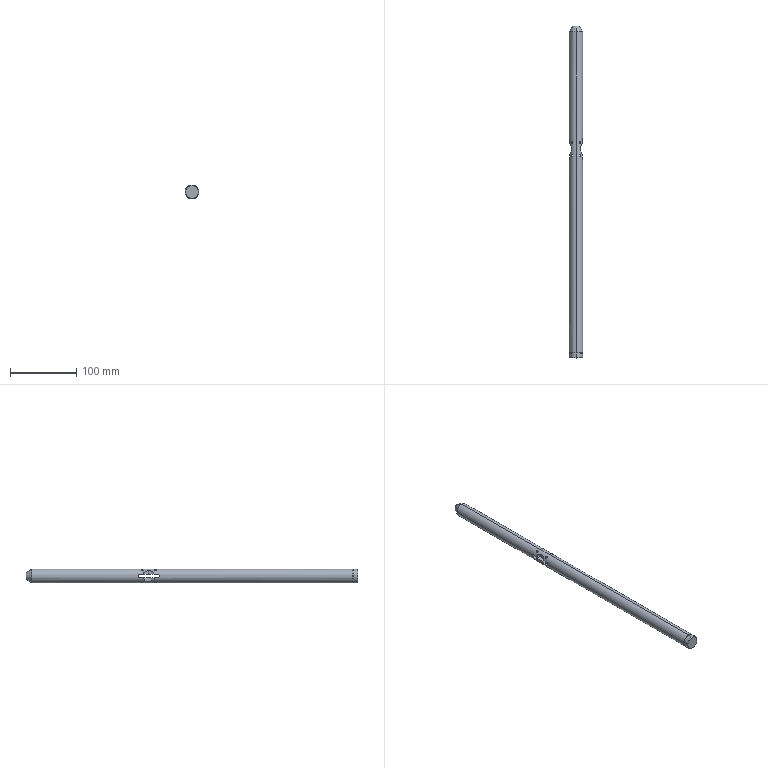Part | STEP file | 06-01 Heat-shrink sleeve shaft | 1 solid | 39 faces | box 20.3 x 500 x 20.3 mm | volume 156269 mm3 | cylinder 27 | plane 8 | cone 4 | commonest cylinder face diameters 3 x16 27 x5 18 x2 20.2 x2 20.3 x2